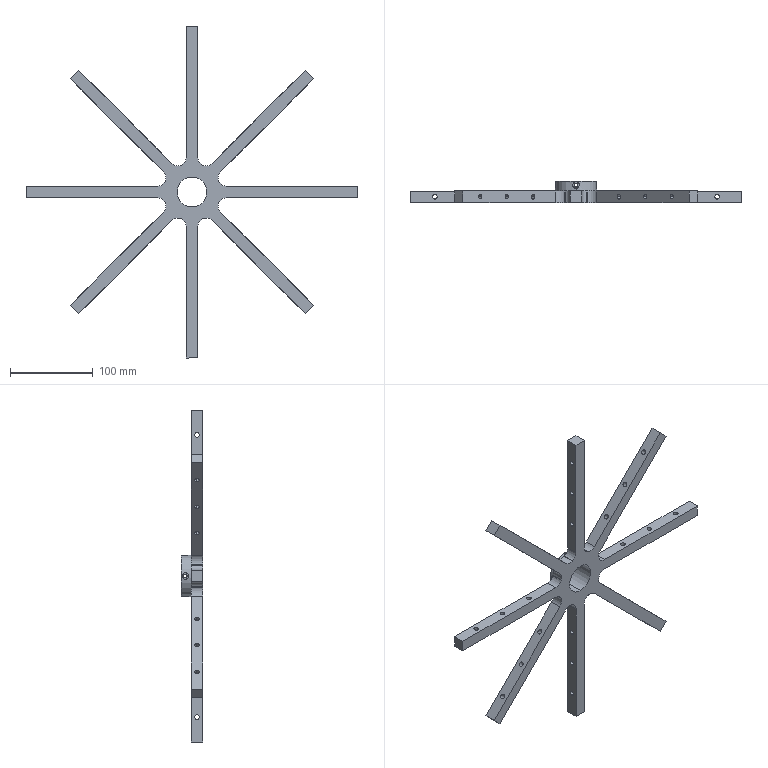Part | SolidWorks | features ICE 6, CirPattern 2, Extrusion 1, Fillet 1 | 1 solid | 125 faces | box 400 x 26 x 400 mm | volume 303636 mm3 | cylinder 94 | plane 31 | commonest cylinder face diameters 5.5 x48 20 x18 4.4 x8 8 x8 70 x8 36 x2